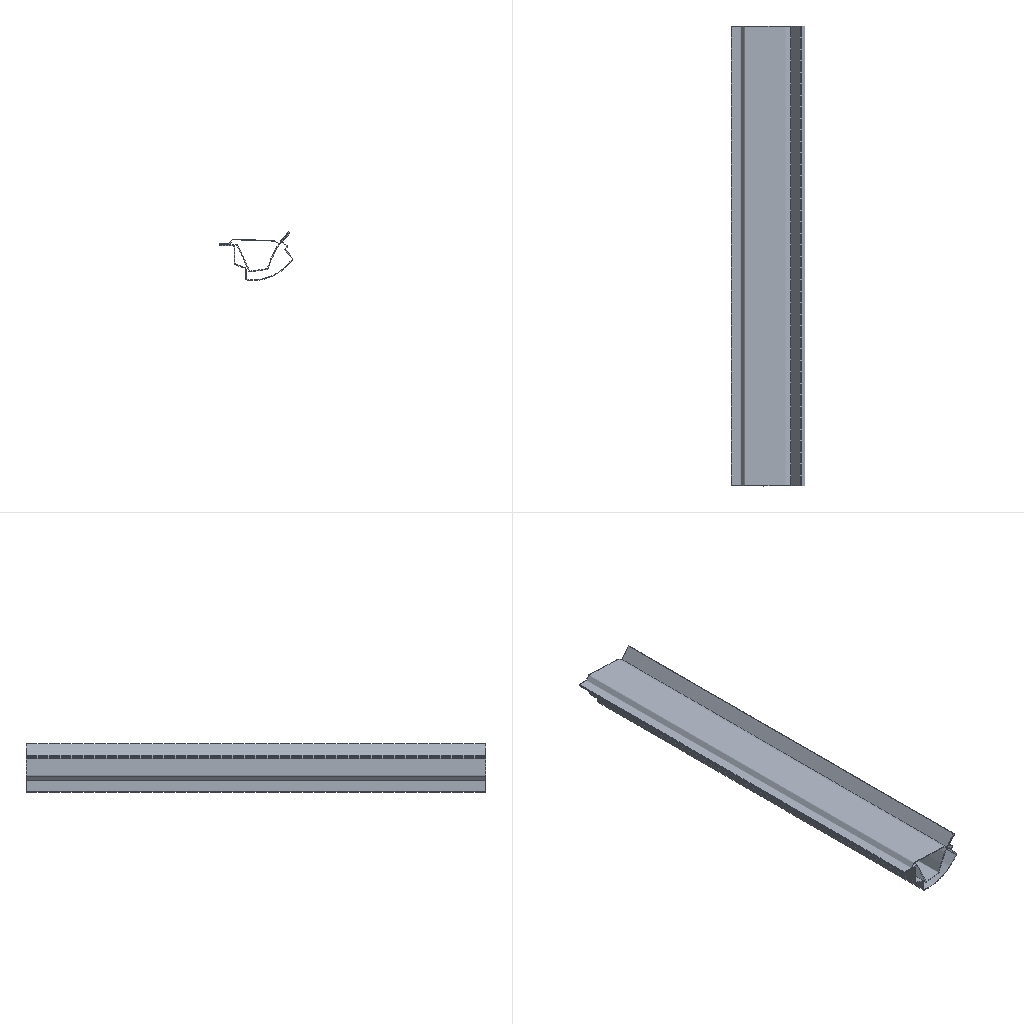Simulation study | ansys workbench
Set-up summary:
category,name,step,type,value,unit,region
solver,ansys_mapdl
solver,version,,,24.2
units,MPA,,stated
analysis,deck,,static,static
load_step,requested,,,1
analysis,nlgeom,,,False
mesh,nodes,,,144934
mesh,elements,,,43680
element_type,ANSYS 186 (type 1),,solid,9520
element_type,ANSYS 186 (type 2),,solid,6160
element_type,ANSYS 186 (type 3),,solid,4620
element_type,ANSYS 174 (type 4),,contact,3080
element_type,ANSYS 170 (type 5),,target,3080
element_type,ANSYS 174 (type 6),,contact,2520
element_type,ANSYS 170 (type 7),,target,2520
element_type,ANSYS 174 (type 8),,contact,2940
element_type,ANSYS 170 (type 9),,target,2940
element_type,ANSYS 154 (type 10),,surface,6300
load,load commands in deck,,count,3
bc,support commands in deck,,count,1
named_set,_FIXEDSU,,component
material,1,,in results
material,2,,in results
material,3,,in results
check,setup vs results,,match,9940 contact/target element(s) of the setup are not in the results: solve.out records that the solver deleted 9940 by its trimming logic; 6300 surface effect element(s) are not in the reader's mesh and were not compared
Ansys APDL input file, long lists of numbers shortened:
/batch
/config,noeldb,1     ! force off writing results to database
*get,_wallstrt,active,,time,wall
! ANSYS input file written by Workbench version 2024 R2
! File used for geometry attach: D:\æ¥å\æ±½è½¦éå¼ºåº¦\é¶ä»¶\zong.stp
/title,wbnew--____ (A5)
! ****** Begin Custom Load Command Snippet ******
/COM, ACT Extensions:
/COM,     LSDYNA, 2024.2
/COM,/COM,     ANSYSMotion, 2024.2
/COM,
! ****** End   Custom Load Command Snippet ******
*DIM,_wb_ProjectScratch_dir,string,248
_wb_ProjectScratch_dir(1) = 'C:\Users\86130\AppData\Local\Temp\WB_86130_53764_4\_ProjectScratch\Scr977A\'
*DIM,_wb_SolverFiles_dir,string,248
_wb_SolverFiles_dir(1) = 'C:\Users\86130\AppData\Local\Temp\WB_86130_53764_4\wbnew_files\dp0\SYS\MECH\'
*DIM,_wb_userfiles_dir,string,248
_wb_userfiles_dir(1) = 'C:\Users\86130\AppData\Local\Temp\WB_86130_53764_4\wbnew_files\user_files\'
/com,--- Data in consistent NMM units. See Solving Units in the help system for more information.
/units,MPA
/nopr
/wb,file,start              !  signify a WB generated input file
/prep7
! Turn off shape checking because checks already performed inside WB mesher.
! See help system for more information.
SHPP,OFF,,NOWARN
/nolist
etcon,set             ! allow ANSYS to choose best KEYOP's for 180x elements, resets any applicable keyopt to MAPDL defaults
/com,*********** Nodes for the whole assembly ***********
nblock,3,,159427
(1i9,3e20.9e3)
   111727     9.497421476E+00     7.000000000E+02     1.200000000E+00
! (144933 more lines like these left out)
-1
/wb,elem,start            !  set before creation of elements
/com,*********** Elements for Body 1 'zong-FreeParts|wai' ***********
et,1,186
keyo,1,2,1          ! set full integration on SOLID186
eblock,19,solid,,9520
(19i9)
        1        1        1        1        0        0        0        0       20        0        1    17499    18342    19037    18197    18055    18895    19038    18198
! (19039 more lines like these left out)
-1
/com,*********** Elements for Body 2 'zong-FreeParts|jia' ***********
et,2,186
keyo,2,2,1          ! set full integration on SOLID186
eblock,19,solid,,6160
(19i9)
        2        2        2        2        0        0        0        0       20        0     9521    78694    80224    80235    79395    79393    80229    80234    79394
! (12319 more lines like these left out)
-1
/com,*********** Elements for Body 3 'zong-FreeParts|nei' ***********
et,3,186
keyo,3,2,1          ! set full integration on SOLID186
eblock,19,solid,,4620
(19i9)
        3        3        3        3        0        0        0        0       20        0    15681   114867   114876   115716   115155   114871   114875   115715   115714
! (9239 more lines like these left out)
-1
/wb,elem,end               !  done creating elements
/com,*********** Send User Defined Coordinate System(s) ***********
csys,0
toffst,273.15,      ! Temperature offset from absolute zero
/com,*********** Set Reference Temperature ***********
tref,22.
/wb,mat,start              !  starting to send materials
/com,*********** Send Materials ***********
Temperature = 'TEMP' ! Temperature
MP,DENS,1,7.85e-09,	! tonne mm^-3
MP,ALPX,1,1.2e-05,	! C^-1
MP,C,1,434000000,	! mm^2 s^-2 C^-1
MP,KXX,1,60.5,	! tonne mm s^-3 C^-1
MP,RSVX,1,0.00017,	! ohm mm
MP,EX,1,200000,	! tonne s^-2 mm^-1
MP,NUXY,1,0.3,
MP,MURX,1,10000,
Temperature = 'TEMP' ! Temperature
MP,DENS,2,7.85e-09,	! tonne mm^-3
MP,ALPX,2,1.2e-05,	! C^-1
MP,C,2,434000000,	! mm^2 s^-2 C^-1
MP,KXX,2,60.5,	! tonne mm s^-3 C^-1
MP,RSVX,2,0.00017,	! ohm mm
MP,EX,2,200000,	! tonne s^-2 mm^-1
MP,NUXY,2,0.3,
MP,MURX,2,10000,
Temperature = 'TEMP' ! Temperature
MP,DENS,3,7.85e-09,	! tonne mm^-3
MP,ALPX,3,1.2e-05,	! C^-1
MP,C,3,434000000,	! mm^2 s^-2 C^-1
MP,KXX,3,60.5,	! tonne mm s^-3 C^-1
MP,RSVX,3,0.00017,	! ohm mm
MP,EX,3,200000,	! tonne s^-2 mm^-1
MP,NUXY,3,0.3,
MP,MURX,3,10000,
/wb,mat,end                !  done sending materials
!************************* Model Summary ********************
!zong-FreeParts|wai,	ç»æé¢,	matid,	1
!zong-FreeParts|jia,	ç»æé¢,	matid,	2
!zong-FreeParts|nei,	ç»æé¢,	matid,	3
!************************* End Model Summary ********************
! get the diagonal of the bounding box. Needed later for other things
*get,_xmin,node,,mnloc,x
*get,_ymin,node,,mnloc,y
*get,_zmin,node,,mnloc,z
*get,_xmax,node,,mxloc,x
*get,_ymax,node,,mxloc,y
*get,_zmax,node,,mxloc,z
_ASMDIAG=(_xmax-_xmin)*(_xmax-_xmin)+(_ymax-_ymin)*(_ymax-_ymin)+(_zmax-_zmin)*(_zmax-_zmin)
_ASMDIAG=SQRT(_ASMDIAG)
/wb,contact,start          !  starting to send contact
/com,*********** Create Contact "½Ó´¥ÇøÓò" ***********
/com,            Real Constant Set For Above Contact Is 5 & 4
*set,tid,5
*set,cid,4
r,tid
r,cid
et,tid,170
et,cid,174
eblock,10,,,1540
(15i9)
    62031        5        5        5        0    18200    18339    18898    18199    65456    65734    65454    65453
! (1539 more lines like these left out)
-1
eblock,10,,,1540
(15i9)
    63571        4        4        4        0    18200    18339    18898    18199    65456    65734    65454    65453
! (1539 more lines like these left out)
-1
eblock,10,,,1540
(15i9)
    65111        4        5        4        0    67740    71973    71834    67739    80525    91909    80523    80521
! (1539 more lines like these left out)
-1
eblock,10,,,1540
(15i9)
    66651        5        4        5        0    67740    71973    71834    67739    80525    91909    80523    80521
! (1539 more lines like these left out)
-1
keyo,cid,8,2               ! auto create asymmetric contact (from Program Controlled setting)
keyo,cid,10,0              ! adjust contact stiffness each NR iteration (from Program Controlled setting)
keyo,cid,12,5              ! bonded always
keyo,cid,18,1              ! small sliding turned on by application
keyo,cid,2,0               ! augmented Lagrange (from Program Controlled setting)
keyo,cid,4,0               ! on Gauss point (from Program Controlled setting)
keyo,cid,9,1               ! ignore initial gaps/penetration
keyo,cid,7,0               ! No Prediction
rmod,tid,3,10.      ! FKN
rmod,tid,5,0.       ! ICONT
rmod,tid,6,0.       ! PINB
rmod,tid,10,0.      ! CNOF
rmod,tid,12,0.      ! FKT
rmod,tid,36,32      ! WB DSID
rmod,cid,3,10.      ! FKN
rmod,cid,5,0.       ! ICONT
rmod,cid,6,0.       ! PINB
rmod,cid,10,0.      ! CNOF
rmod,cid,12,0.      ! FKT
rmod,cid,36,32      ! WB DSID
/com,*********** Create Contact "½Ó´¥ÇøÓò 2" ***********
/com,            Real Constant Set For Above Contact Is 7 & 6
*set,tid,7
*set,cid,6
r,tid
r,cid
et,tid,170
et,cid,174
eblock,10,,,1260
(15i9)
    68191        7        7        7        0    18200    18339    18898    18199    65456    65734    65454    65453
! (1259 more lines like these left out)
-1
eblock,10,,,1260
(15i9)
    69451        6        6        6        0    18200    18339    18898    18199    65456    65734    65454    65453
! (1259 more lines like these left out)
-1
eblock,10,,,1260
(15i9)
    70711        6        7        6        0   120894   111935   111795   120755   122044   121484   121486   143959
! (1259 more lines like these left out)
-1
eblock,10,,,1260
(15i9)
    71971        7        6        7        0   120894   111935   111795   120755   122044   121484   121486   143959
! (1259 more lines like these left out)
-1
keyo,cid,8,2               ! auto create asymmetric contact (from Program Controlled setting)
keyo,cid,10,0              ! adjust contact stiffness each NR iteration (from Program Controlled setting)
keyo,cid,12,5              ! bonded always
keyo,cid,18,1              ! small sliding turned on by application
keyo,cid,2,0               ! augmented Lagrange (from Program Controlled setting)
keyo,cid,4,0               ! on Gauss point (from Program Controlled setting)
keyo,cid,9,1               ! ignore initial gaps/penetration
keyo,cid,7,0               ! No Prediction
rmod,tid,3,10.      ! FKN
rmod,tid,5,0.       ! ICONT
rmod,tid,6,0.       ! PINB
rmod,tid,10,0.      ! CNOF
rmod,tid,12,0.      ! FKT
rmod,tid,36,35      ! WB DSID
rmod,cid,3,10.      ! FKN
rmod,cid,5,0.       ! ICONT
rmod,cid,6,0.       ! PINB
rmod,cid,10,0.      ! CNOF
rmod,cid,12,0.      ! FKT
rmod,cid,36,35      ! WB DSID
/com,*********** Create Contact "½Ó´¥ÇøÓò 3" ***********
/com,            Real Constant Set For Above Contact Is 9 & 8
*set,tid,9
*set,cid,8
r,tid
r,cid
et,tid,170
et,cid,174
eblock,10,,,1540
(15i9)
    73231        9        9        9        0    73515    72814    73513    73514    94564    94563    95955    95956
! (1539 more lines like these left out)
-1
eblock,10,,,1540
(15i9)
    74771        8        8        8        0    73515    72814    73513    73514    94564    94563    95955    95956
! (1539 more lines like these left out)
-1
eblock,10,,,1400
(15i9)
    76311        8        9        8        0   120894   111935   111795   120755   122044   121484   121486   143959
! (1399 more lines like these left out)
-1
eblock,10,,,1400
(15i9)
    77711        9        8        9        0   120894   111935   111795   120755   122044   121484   121486   143959
! (1399 more lines like these left out)
-1
keyo,cid,8,2               ! auto create asymmetric contact (from Program Controlled setting)
keyo,cid,10,0              ! adjust contact stiffness each NR iteration (from Program Controlled setting)
keyo,cid,12,5              ! bonded always
keyo,cid,18,1              ! small sliding turned on by application
keyo,cid,2,0               ! augmented Lagrange (from Program Controlled setting)
keyo,cid,4,0               ! on Gauss point (from Program Controlled setting)
keyo,cid,9,1               ! ignore initial gaps/penetration
keyo,cid,7,0               ! No Prediction
rmod,tid,3,10.      ! FKN
rmod,tid,5,0.       ! ICONT
rmod,tid,6,0.       ! PINB
rmod,tid,10,0.      ! CNOF
rmod,tid,12,0.      ! FKT
rmod,tid,36,38      ! WB DSID
rmod,cid,3,10.      ! FKN
rmod,cid,5,0.       ! ICONT
rmod,cid,6,0.       ! PINB
rmod,cid,10,0.      ! CNOF
rmod,cid,12,0.      ! FKT
rmod,cid,36,38      ! WB DSID
nsel,all
esel,all
/wb,contact,end            !  done creating contacts
/golist
/wb,load,start             !  starting to send loads
/com,*********** Fixed Supports ***********
CMBLOCK,_FIXEDSU,NODE,     1468
(8i10)
         1         2         3         4         5         6         7         8
! (183 more lines like these left out)
cmsel,s,_FIXEDSU
d,all,all
nsel,all
/com,*********** Define Force Using Surface Effect Elements ***********
local,12,0,0.,0.,0.,0.,0.,0.
csys,0
et,10,154
mat,10
eblock,10,,,6300
(15i9)
    79111       10       10       10       12      701    16659       16      134    21488    19502    19501    19793
! (6299 more lines like these left out)
-1
esel,s,type,,10
keyop,10,2,1        ! Apply load in local coordinate system
keyop,10,7,1        ! Use original area so load is constant in large deformation
esel,all
/gst,on,on
fini
*get,_numnode,node,0,count
*get,_numelem,elem,0,count
*get, _MAXELEMNUM, elem, 0, NUM, MAX
*get, _MAXNODENUM, node, 0, NUM, MAX
*get, _MAXELEMTYPE, etyp, 0, NUM, MAX
*get, _MAXREALCONST, rcon, 0, NUM, MAX
/go
/wb,load,end               !  done creating loads
/com,--- Number of total nodes = %_numnode%
/com,--- Number of contact elements = 23380
/com,--- Number of spring elements = 0
/com,--- Number of bearing elements = 0
/com,--- Number of solid elements = 20300
/com,--- Number of condensed parts = 0
/com,--- Number of total elements = %_numelem%
*get,_wallbsol,active,,time,wall
/com,****************************************************************************
/com,*************************    SOLUTION       ********************************
/com,****************************************************************************
/solu
antype,0                   ! static analysis
_thickRatio=  0     ! Ratio of thick parts in the model
eqsl,sparse,,,,,1
cntr,print,1               ! print out contact info and also make no initial contact an error
cncheck,dmp		!	Enable program controlled contact splitting for distributed memory parallel run
dmpoption,emat,no             ! Don't combine emat file for DANSYS
dmpoption,esav,no             ! Don't combine esav file for DANSYS
nldiag,cont,iter           ! print out contact info each equilibrium iteration
rescontrol,,none                 ! Do not keep any restart files
/com,****************************************************
/com,******************* SOLVE FOR LS 1 OF 1 ****************
esel,s,type,,10
nsle
sfe,all,1,pres,1,0.
sfe,all,2,pres,1,0.
sfe,all,3,pres,1,0.154
nsel,all
esel,all
/nopr
/gopr
nsub,1,1,1
time,1.
outres,erase
outres,all,none
outres,nsol,all,
outres,rsol,all
outres,eangl,all
outres,etmp,all
outres,veng,all
outres,strs,all,
outres,epel,all,
outres,eppl,all,
outres,cont,all,
! *********** WB SOLVE COMMAND ***********
! check interactive state
*get,ANSINTER_,active,,int
*if,ANSINTER_,ne,0,then
/eof
*endif
solve
/com *************** Write FE CONNECTORS *********
CEWRITE,file,ce,,INTE
/com,****************************************************
/com,*************** FINISHED SOLVE FOR LS 1 *************
*get,_wallasol,active,,time,wall
/nopr
*get,_numnode,node,0,count
*get,_numelem,elem,0,count
*get, _MAXELEMNUM, elem, 0, NUM, MAX
*get, _MAXNODENUM, node, 0, NUM, MAX,,,INTERNAL
*get, _MAXELEMTYPE, etyp, 0, NUM, MAX
*get, _MAXREALCONST, rcon, 0, NUM, MAX
*get,_NSOLTHREADS,active,0,ntfs
*get,_NSOLPROCESSES,active,0,npfs
/gopr
/post1
xmlo,ENCODING,ISO-8859-1
xmlo,parm
/xml,parm,xml
fini
/gopr
*get,_walldone,active,,time,wall
_preptime=(_wallbsol-_wallstrt)*3600
_solvtime=(_wallasol-_wallbsol)*3600
_posttime=(_walldone-_wallasol)*3600
_totaltim=(_walldone-_wallstrt)*3600
*get,_dlbratio,active,0,solu,dlbr
*get,_combtime,active,0,solu,comb
*get,_ssmode,active,0,solu,ssmm
*get,_ndofs,active,0,solu,ndof
*get,_sol_end_time,active,0,set,time
*if,_sol_end_time,eq,1.,then
/fclean				!clean distributed files
*endif
/com,--- Total number of nodes = %_numnode%
/com,--- Total number of elements = %_numelem%
/com,--- Element load balance ratio = %_dlbratio%
/com,--- Time to combine distributed files = %_combtime%
/com,--- Sparse memory mode = %_ssmode%
/com,--- Number of DOF = %_ndofs%
/wb,file,end               ! done with WB generated input
Results summary:
result,analysis,,,static
result,last_loadstep,,,1
result,primary field,,,displacement
result,reaction total,1,FX,-1.5e-05,N
result,reaction total,1,FY,-8.4e-05,N
result,reaction total,1,FZ,-20580,N
result,mass,,,0.002817,"NMM: mm, ton, N, s, mV, mA, degC"